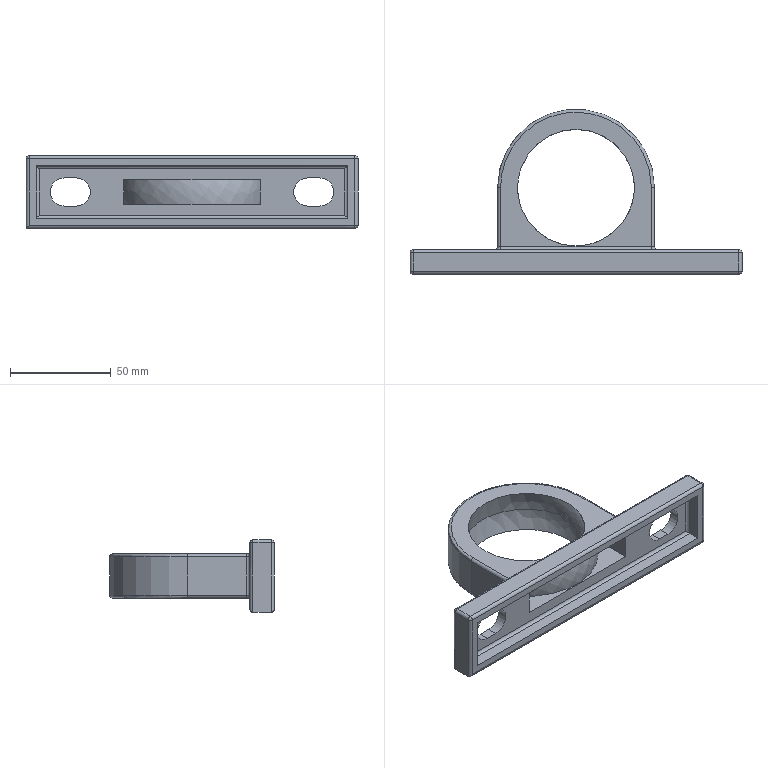Part | SolidWorks | features BaseBody 1 | 1 solid | 66 faces | volume 77095 mm3 | cylinder 28 | plane 23 | spline 15 | commonest cylinder face diameters 3 x23 14 x4 78 x1